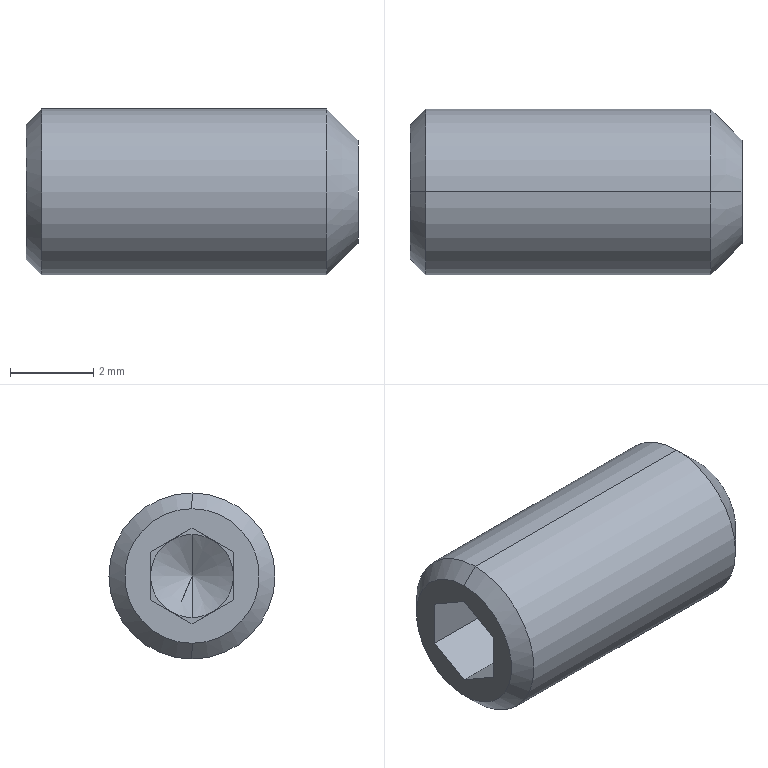Part | SolidWorks | features BaseBody 1 | 1 solid | 22 faces | box 8 x 4 x 4 mm | volume 90.792 mm3 | plane 14 | cone 6 | cylinder 2 | commonest cylinder face diameters 4 x2
STEP:
#1=CARTESIAN_POINT('',(2.077,0.,0.));
#2=VERTEX_POINT('',#1);
#3=CARTESIAN_POINT('',(1.5,0.,1.));
#4=VERTEX_POINT('',#3);
#5=CARTESIAN_POINT('',(2.077,0.,0.));
#6=DIRECTION('',(-0.5,0.,0.866));
#7=VECTOR('',#6,1000.);
#8=LINE('',#5,#7);
#9=EDGE_CURVE('',#2,#4,#8,.T.);
#10=ORIENTED_EDGE('',*,*,#9,.F.);
#11=CARTESIAN_POINT('',(1.5,0.,-1.));
#12=VERTEX_POINT('',#11);
#13=CARTESIAN_POINT('',(2.077,0.,0.));
#14=DIRECTION('',(-0.5,0.,-0.866));
#15=VECTOR('',#14,1000.);
#16=LINE('',#13,#15);
#17=EDGE_CURVE('',#2,#12,#16,.T.);
#18=ORIENTED_EDGE('',*,*,#17,.T.);
#19=CARTESIAN_POINT('',(1.5,-0.5,-0.866));
#20=VERTEX_POINT('',#19);
#21=CARTESIAN_POINT('',(1.5,0.,0.));
#22=DIRECTION('',(-1.,0.,0.));
#23=DIRECTION('',(0.,0.,1.));
#24=AXIS2_PLACEMENT_3D('',#21,#22,#23);
#25=CIRCLE('',#24,1.);
#26=EDGE_CURVE('',#12,#20,#25,.T.);
#27=ORIENTED_EDGE('',*,*,#26,.T.);
#28=CARTESIAN_POINT('',(1.5,-1.,0.));
#29=VERTEX_POINT('',#28);
#30=CARTESIAN_POINT('',(1.5,0.,0.));
#31=DIRECTION('',(-1.,0.,0.));
#32=DIRECTION('',(0.,0.,1.));
#33=AXIS2_PLACEMENT_3D('',#30,#31,#32);
#34=CIRCLE('',#33,1.);
#35=EDGE_CURVE('',#20,#29,#34,.T.);
#36=ORIENTED_EDGE('',*,*,#35,.T.);
#37=CARTESIAN_POINT('',(1.5,-0.5,0.866));
#38=VERTEX_POINT('',#37);
#39=CARTESIAN_POINT('',(1.5,0.,0.));
#40=DIRECTION('',(-1.,0.,0.));
#41=DIRECTION('',(0.,0.,1.));
#42=AXIS2_PLACEMENT_3D('',#39,#40,#41);
#43=CIRCLE('',#42,1.);
#44=EDGE_CURVE('',#29,#38,#43,.T.);
#45=ORIENTED_EDGE('',*,*,#44,.T.);
#46=CARTESIAN_POINT('',(1.5,0.,0.));
#47=DIRECTION('',(-1.,0.,0.));
#48=DIRECTION('',(0.,0.,1.));
#49=AXIS2_PLACEMENT_3D('',#46,#47,#48);
#50=CIRCLE('',#49,1.);
#51=EDGE_CURVE('',#38,#4,#50,.T.);
#52=ORIENTED_EDGE('',*,*,#51,.T.);
#53=EDGE_LOOP('',(#10,#18,#27,#36,#45,#52));
#54=FACE_OUTER_BOUND('',#53,.T.);
#55=CARTESIAN_POINT('',(-997.923,0.,0.));
#56=DIRECTION('',(-1.,0.,0.));
#57=DIRECTION('',(0.,0.,1.));
#58=AXIS2_PLACEMENT_3D('',#55,#56,#57);
#59=CONICAL_SURFACE('',#58,1732.051,1.047);
#60=ADVANCED_FACE('',(#54),#59,.F.);
#61=CARTESIAN_POINT('',(0.,0.,1.621));
#62=VERTEX_POINT('',#61);
#63=CARTESIAN_POINT('',(0.,0.,-1.621));
#64=VERTEX_POINT('',#63);
#65=CARTESIAN_POINT('',(0.,0.,0.));
#66=DIRECTION('',(-1.,0.,0.));
#67=DIRECTION('',(0.,0.,1.));
#68=AXIS2_PLACEMENT_3D('',#65,#66,#67);
#69=CIRCLE('',#68,1.621);
#70=EDGE_CURVE('',#62,#64,#69,.T.);
#71=ORIENTED_EDGE('',*,*,#70,.F.);
#72=CARTESIAN_POINT('',(0.379,0.,2.));
#73=VERTEX_POINT('',#72);
#74=CARTESIAN_POINT('',(0.379,0.,2.));
#75=DIRECTION('',(0.7071,0.,0.7071));
#76=VECTOR('',#75,1000.);
#77=LINE('',#74,#76);
#78=EDGE_CURVE('',#62,#73,#77,.T.);
#79=ORIENTED_EDGE('',*,*,#78,.T.);
#80=CARTESIAN_POINT('',(0.379,0.,-2.));
#81=VERTEX_POINT('',#80);
#82=CARTESIAN_POINT('',(0.379,0.,0.));
#83=DIRECTION('',(-1.,0.,0.));
#84=DIRECTION('',(0.,0.,1.));
#85=AXIS2_PLACEMENT_3D('',#82,#83,#84);
#86=CIRCLE('',#85,2.);
#87=EDGE_CURVE('',#73,#81,#86,.T.);
#88=ORIENTED_EDGE('',*,*,#87,.T.);
#89=CARTESIAN_POINT('',(0.379,0.,-2.));
#90=DIRECTION('',(0.7071,0.,-0.7071));
#91=VECTOR('',#90,1000.);
#92=LINE('',#89,#91);
#93=EDGE_CURVE('',#64,#81,#92,.T.);
#94=ORIENTED_EDGE('',*,*,#93,.F.);
#95=EDGE_LOOP('',(#71,#79,#88,#94));
#96=FACE_OUTER_BOUND('',#95,.T.);
#97=CARTESIAN_POINT('',(0.379,0.,0.));
#98=DIRECTION('',(1.,0.,0.));
#99=DIRECTION('',(0.,0.,-1.));
#100=AXIS2_PLACEMENT_3D('',#97,#98,#99);
#101=CONICAL_SURFACE('',#100,2.,0.7854);
#102=ADVANCED_FACE('',(#96),#101,.T.);
#103=CARTESIAN_POINT('',(7.25,0.,2.));
#104=VERTEX_POINT('',#103);
#105=CARTESIAN_POINT('',(7.25,0.,-2.));
#106=VERTEX_POINT('',#105);
#107=CARTESIAN_POINT('',(7.25,0.,0.));
#108=DIRECTION('',(-1.,0.,0.));
#109=DIRECTION('',(0.,0.,1.));
#110=AXIS2_PLACEMENT_3D('',#107,#108,#109);
#111=CIRCLE('',#110,2.);
#112=EDGE_CURVE('',#104,#106,#111,.T.);
#113=ORIENTED_EDGE('',*,*,#112,.T.);
#114=CARTESIAN_POINT('',(-10.745,0.,-2.));
#115=DIRECTION('',(-1.,0.,0.));
#116=VECTOR('',#115,1000.);
#117=LINE('',#114,#116);
#118=EDGE_CURVE('',#106,#81,#117,.T.);
#119=ORIENTED_EDGE('',*,*,#118,.T.);
#120=ORIENTED_EDGE('',*,*,#87,.F.);
#121=CARTESIAN_POINT('',(-10.745,0.,2.));
#122=DIRECTION('',(-1.,0.,0.));
#123=VECTOR('',#122,1000.);
#124=LINE('',#121,#123);
#125=EDGE_CURVE('',#104,#73,#124,.T.);
#126=ORIENTED_EDGE('',*,*,#125,.F.);
#127=EDGE_LOOP('',(#113,#119,#120,#126));
#128=FACE_OUTER_BOUND('',#127,.T.);
#129=CARTESIAN_POINT('',(-10.745,0.,0.));
#130=DIRECTION('',(-1.,0.,0.));
#131=DIRECTION('',(0.,0.,1.));
#132=AXIS2_PLACEMENT_3D('',#129,#130,#131);
#133=CYLINDRICAL_SURFACE('',#132,2.);
#134=ADVANCED_FACE('',(#128),#133,.T.);
#135=CARTESIAN_POINT('',(8.,0.,1.25));
#136=VERTEX_POINT('',#135);
#137=CARTESIAN_POINT('',(8.,0.,-1.25));
#138=VERTEX_POINT('',#137);
#139=CARTESIAN_POINT('',(8.,0.,0.));
#140=DIRECTION('',(-1.,0.,0.));
#141=DIRECTION('',(0.,0.,1.));
#142=AXIS2_PLACEMENT_3D('',#139,#140,#141);
#143=CIRCLE('',#142,1.25);
#144=EDGE_CURVE('',#136,#138,#143,.T.);
#145=ORIENTED_EDGE('',*,*,#144,.T.);
#146=CARTESIAN_POINT('',(8.,0.,-1.25));
#147=DIRECTION('',(-0.7071,0.,-0.7071));
#148=VECTOR('',#147,1000.);
#149=LINE('',#146,#148);
#150=EDGE_CURVE('',#138,#106,#149,.T.);
#151=ORIENTED_EDGE('',*,*,#150,.T.);
#152=ORIENTED_EDGE('',*,*,#112,.F.);
#153=CARTESIAN_POINT('',(8.,0.,1.25));
#154=DIRECTION('',(-0.7071,0.,0.7071));
#155=VECTOR('',#154,1000.);
#156=LINE('',#153,#155);
#157=EDGE_CURVE('',#136,#104,#156,.T.);
#158=ORIENTED_EDGE('',*,*,#157,.F.);
#159=EDGE_LOOP('',(#145,#151,#152,#158));
#160=FACE_OUTER_BOUND('',#159,.T.);
#161=CARTESIAN_POINT('',(8.,0.,0.));
#162=DIRECTION('',(-1.,0.,0.));
#163=DIRECTION('',(0.,0.,1.));
#164=AXIS2_PLACEMENT_3D('',#161,#162,#163);
#165=CONICAL_SURFACE('',#164,1.25,0.7854);
#166=ADVANCED_FACE('',(#160),#165,.T.);
#167=CARTESIAN_POINT('',(1.5,0.5,0.866));
#168=VERTEX_POINT('',#167);
#169=CARTESIAN_POINT('',(1.5,1.,0.));
#170=VERTEX_POINT('',#169);
#171=CARTESIAN_POINT('',(1.5,0.,0.));
#172=DIRECTION('',(-1.,0.,0.));
#173=DIRECTION('',(0.,0.,1.));
#174=AXIS2_PLACEMENT_3D('',#171,#172,#173);
#175=CIRCLE('',#174,1.);
#176=EDGE_CURVE('',#168,#170,#175,.T.);
#177=ORIENTED_EDGE('',*,*,#176,.F.);
#178=CARTESIAN_POINT('',(1.5,1.,0.5774));
#179=VERTEX_POINT('',#178);
#180=CARTESIAN_POINT('',(1.5,0.,1.155));
#181=DIRECTION('',(0.,0.866,-0.5));
#182=VECTOR('',#181,1000.);
#183=LINE('',#180,#182);
#184=EDGE_CURVE('',#168,#179,#183,.T.);
#185=ORIENTED_EDGE('',*,*,#184,.T.);
#186=CARTESIAN_POINT('',(1.5,1.,0.5774));
#187=DIRECTION('',(0.,0.,-1.));
#188=VECTOR('',#187,1000.);
#189=LINE('',#186,#188);
#190=EDGE_CURVE('',#179,#170,#189,.T.);
#191=ORIENTED_EDGE('',*,*,#190,.T.);
#192=EDGE_LOOP('',(#177,#185,#191));
#193=FACE_OUTER_BOUND('',#192,.T.);
#194=CARTESIAN_POINT('',(1.5,-1.,0.5774));
#195=DIRECTION('',(1.,0.,0.));
#196=DIRECTION('',(0.,1.,0.));
#197=AXIS2_PLACEMENT_3D('',#194,#195,#196);
#198=PLANE('',#197);
#199=ADVANCED_FACE('',(#193),#198,.F.);
#200=CARTESIAN_POINT('',(1.5,0.5,-0.866));
#201=VERTEX_POINT('',#200);
#202=CARTESIAN_POINT('',(1.5,0.,0.));
#203=DIRECTION('',(-1.,0.,0.));
#204=DIRECTION('',(0.,0.,1.));
#205=AXIS2_PLACEMENT_3D('',#202,#203,#204);
#206=CIRCLE('',#205,1.);
#207=EDGE_CURVE('',#170,#201,#206,.T.);
#208=ORIENTED_EDGE('',*,*,#207,.F.);
#209=CARTESIAN_POINT('',(1.5,1.,-0.5774));
#210=VERTEX_POINT('',#209);
#211=CARTESIAN_POINT('',(1.5,1.,0.5774));
#212=DIRECTION('',(0.,0.,-1.));
#213=VECTOR('',#212,1000.);
#214=LINE('',#211,#213);
#215=EDGE_CURVE('',#170,#210,#214,.T.);
#216=ORIENTED_EDGE('',*,*,#215,.T.);
#217=CARTESIAN_POINT('',(1.5,1.,-0.5774));
#218=DIRECTION('',(0.,-0.866,-0.5));
#219=VECTOR('',#218,1000.);
#220=LINE('',#217,#219);
#221=EDGE_CURVE('',#210,#201,#220,.T.);
#222=ORIENTED_EDGE('',*,*,#221,.T.);
#223=EDGE_LOOP('',(#208,#216,#222));
#224=FACE_OUTER_BOUND('',#223,.T.);
#225=CARTESIAN_POINT('',(1.5,-1.,0.5774));
#226=DIRECTION('',(1.,0.,0.));
#227=DIRECTION('',(0.,1.,0.));
#228=AXIS2_PLACEMENT_3D('',#225,#226,#227);
#229=PLANE('',#228);
#230=ADVANCED_FACE('',(#224),#229,.F.);
#231=CARTESIAN_POINT('',(1.5,0.,0.));
#232=DIRECTION('',(-1.,0.,0.));
#233=DIRECTION('',(0.,0.,1.));
#234=AXIS2_PLACEMENT_3D('',#231,#232,#233);
#235=CIRCLE('',#234,1.);
#236=EDGE_CURVE('',#201,#12,#235,.T.);
#237=ORIENTED_EDGE('',*,*,#236,.F.);
#238=CARTESIAN_POINT('',(1.5,0.,-1.155));
#239=VERTEX_POINT('',#238);
#240=CARTESIAN_POINT('',(1.5,1.,-0.5774));
#241=DIRECTION('',(0.,-0.866,-0.5));
#242=VECTOR('',#241,1000.);
#243=LINE('',#240,#242);
#244=EDGE_CURVE('',#201,#239,#243,.T.);
#245=ORIENTED_EDGE('',*,*,#244,.T.);
#246=CARTESIAN_POINT('',(1.5,0.,-1.155));
#247=DIRECTION('',(0.,-0.866,0.5));
#248=VECTOR('',#247,1000.);
#249=LINE('',#246,#248);
#250=EDGE_CURVE('',#239,#20,#249,.T.);
#251=ORIENTED_EDGE('',*,*,#250,.T.);
#252=ORIENTED_EDGE('',*,*,#26,.F.);
#253=EDGE_LOOP('',(#237,#245,#251,#252));
#254=FACE_OUTER_BOUND('',#253,.T.);
#255=CARTESIAN_POINT('',(1.5,-1.,0.5774));
#256=DIRECTION('',(1.,0.,0.));
#257=DIRECTION('',(0.,1.,0.));
#258=AXIS2_PLACEMENT_3D('',#255,#256,#257);
#259=PLANE('',#258);
#260=ADVANCED_FACE('',(#254),#259,.F.);
#261=ORIENTED_EDGE('',*,*,#35,.F.);
#262=CARTESIAN_POINT('',(1.5,-1.,-0.5774));
#263=VERTEX_POINT('',#262);
#264=CARTESIAN_POINT('',(1.5,0.,-1.155));
#265=DIRECTION('',(0.,-0.866,0.5));
#266=VECTOR('',#265,1000.);
#267=LINE('',#264,#266);
#268=EDGE_CURVE('',#20,#263,#267,.T.);
#269=ORIENTED_EDGE('',*,*,#268,.T.);
#270=CARTESIAN_POINT('',(1.5,-1.,-0.5774));
#271=DIRECTION('',(0.,0.,1.));
#272=VECTOR('',#271,1000.);
#273=LINE('',#270,#272);
#274=EDGE_CURVE('',#263,#29,#273,.T.);
#275=ORIENTED_EDGE('',*,*,#274,.T.);
#276=EDGE_LOOP('',(#261,#269,#275));
#277=FACE_OUTER_BOUND('',#276,.T.);
#278=CARTESIAN_POINT('',(1.5,-1.,0.5774));
#279=DIRECTION('',(1.,0.,0.));
#280=DIRECTION('',(0.,1.,0.));
#281=AXIS2_PLACEMENT_3D('',#278,#279,#280);
#282=PLANE('',#281);
#283=ADVANCED_FACE('',(#277),#282,.F.);
#284=ORIENTED_EDGE('',*,*,#44,.F.);
#285=CARTESIAN_POINT('',(1.5,-1.,0.5774));
#286=VERTEX_POINT('',#285);
#287=CARTESIAN_POINT('',(1.5,-1.,-0.5774));
#288=DIRECTION('',(0.,0.,1.));
#289=VECTOR('',#288,1000.);
#290=LINE('',#287,#289);
#291=EDGE_CURVE('',#29,#286,#290,.T.);
#292=ORIENTED_EDGE('',*,*,#291,.T.);
#293=CARTESIAN_POINT('',(1.5,-1.,0.5774));
#294=DIRECTION('',(0.,0.866,0.5));
#295=VECTOR('',#294,1000.);
#296=LINE('',#293,#295);
#297=EDGE_CURVE('',#286,#38,#296,.T.);
#298=ORIENTED_EDGE('',*,*,#297,.T.);
#299=EDGE_LOOP('',(#284,#292,#298));
#300=FACE_OUTER_BOUND('',#299,.T.);
#301=CARTESIAN_POINT('',(1.5,-1.,0.5774));
#302=DIRECTION('',(1.,0.,0.));
#303=DIRECTION('',(0.,1.,0.));
#304=AXIS2_PLACEMENT_3D('',#301,#302,#303);
#305=PLANE('',#304);
#306=ADVANCED_FACE('',(#300),#305,.F.);
#307=ORIENTED_EDGE('',*,*,#51,.F.);
#308=CARTESIAN_POINT('',(1.5,0.,1.155));
#309=VERTEX_POINT('',#308);
#310=CARTESIAN_POINT('',(1.5,-1.,0.5774));
#311=DIRECTION('',(0.,0.866,0.5));
#312=VECTOR('',#311,1000.);
#313=LINE('',#310,#312);
#314=EDGE_CURVE('',#38,#309,#313,.T.);
#315=ORIENTED_EDGE('',*,*,#314,.T.);
#316=CARTESIAN_POINT('',(1.5,0.,1.155));
#317=DIRECTION('',(0.,0.866,-0.5));
#318=VECTOR('',#317,1000.);
#319=LINE('',#316,#318);
#320=EDGE_CURVE('',#309,#168,#319,.T.);
#321=ORIENTED_EDGE('',*,*,#320,.T.);
#322=CARTESIAN_POINT('',(1.5,0.,0.));
#323=DIRECTION('',(-1.,0.,0.));
#324=DIRECTION('',(0.,0.,1.));
#325=AXIS2_PLACEMENT_3D('',#322,#323,#324);
#326=CIRCLE('',#325,1.);
#327=EDGE_CURVE('',#4,#168,#326,.T.);
#328=ORIENTED_EDGE('',*,*,#327,.F.);
#329=EDGE_LOOP('',(#307,#315,#321,#328));
#330=FACE_OUTER_BOUND('',#329,.T.);
#331=CARTESIAN_POINT('',(1.5,-1.,0.5774));
#332=DIRECTION('',(1.,0.,0.));
#333=DIRECTION('',(0.,1.,0.));
#334=AXIS2_PLACEMENT_3D('',#331,#332,#333);
#335=PLANE('',#334);
#336=ADVANCED_FACE('',(#330),#335,.F.);
#337=CARTESIAN_POINT('',(0.,0.,1.155));
#338=VERTEX_POINT('',#337);
#339=CARTESIAN_POINT('',(0.,1.,0.5774));
#340=VERTEX_POINT('',#339);
#341=CARTESIAN_POINT('',(0.,0.,1.155));
#342=DIRECTION('',(0.,0.866,-0.5));
#343=VECTOR('',#342,1000.);
#344=LINE('',#341,#343);
#345=EDGE_CURVE('',#338,#340,#344,.T.);
#346=ORIENTED_EDGE('',*,*,#345,.F.);
#347=CARTESIAN_POINT('',(0.,-1.,0.5774));
#348=VERTEX_POINT('',#347);
#349=CARTESIAN_POINT('',(0.,-1.,0.5774));
#350=DIRECTION('',(0.,0.866,0.5));
#351=VECTOR('',#350,1000.);
#352=LINE('',#349,#351);
#353=EDGE_CURVE('',#348,#338,#352,.T.);
#354=ORIENTED_EDGE('',*,*,#353,.F.);
#355=CARTESIAN_POINT('',(0.,-1.,-0.5774));
#356=VERTEX_POINT('',#355);
#357=CARTESIAN_POINT('',(0.,-1.,-0.5774));
#358=DIRECTION('',(0.,0.,1.));
#359=VECTOR('',#358,1000.);
#360=LINE('',#357,#359);
#361=EDGE_CURVE('',#356,#348,#360,.T.);
#362=ORIENTED_EDGE('',*,*,#361,.F.);
#363=CARTESIAN_POINT('',(0.,0.,-1.155));
#364=VERTEX_POINT('',#363);
#365=CARTESIAN_POINT('',(0.,0.,-1.155));
#366=DIRECTION('',(0.,-0.866,0.5));
#367=VECTOR('',#366,1000.);
#368=LINE('',#365,#367);
#369=EDGE_CURVE('',#364,#356,#368,.T.);
#370=ORIENTED_EDGE('',*,*,#369,.F.);
#371=CARTESIAN_POINT('',(0.,1.,-0.5774));
#372=VERTEX_POINT('',#371);
#373=CARTESIAN_POINT('',(0.,1.,-0.5774));
#374=DIRECTION('',(0.,-0.866,-0.5));
#375=VECTOR('',#374,1000.);
#376=LINE('',#373,#375);
#377=EDGE_CURVE('',#372,#364,#376,.T.);
#378=ORIENTED_EDGE('',*,*,#377,.F.);
#379=CARTESIAN_POINT('',(0.,1.,0.5774));
#380=DIRECTION('',(0.,0.,-1.));
#381=VECTOR('',#380,1000.);
#382=LINE('',#379,#381);
#383=EDGE_CURVE('',#340,#372,#382,.T.);
#384=ORIENTED_EDGE('',*,*,#383,.F.);
#385=EDGE_LOOP('',(#346,#354,#362,#370,#378,#384));
#386=FACE_BOUND('',#385,.T.);
#387=CARTESIAN_POINT('',(0.,0.,0.));
#388=DIRECTION('',(-1.,0.,0.));
#389=DIRECTION('',(0.,0.,1.));
#390=AXIS2_PLACEMENT_3D('',#387,#388,#389);
#391=CIRCLE('',#390,1.621);
#392=EDGE_CURVE('',#64,#62,#391,.T.);
#393=ORIENTED_EDGE('',*,*,#392,.T.);
#394=ORIENTED_EDGE('',*,*,#70,.T.);
#395=EDGE_LOOP('',(#393,#394));
#396=FACE_OUTER_BOUND('',#395,.T.);
#397=CARTESIAN_POINT('',(0.,1.621,0.));
#398=DIRECTION('',(1.,0.,0.));
#399=DIRECTION('',(0.,1.,0.));
#400=AXIS2_PLACEMENT_3D('',#397,#398,#399);
#401=PLANE('',#400);
#402=ADVANCED_FACE('',(#386,#396),#401,.F.);
#403=ORIENTED_EDGE('',*,*,#144,.F.);
#404=CARTESIAN_POINT('',(8.,0.,0.));
#405=DIRECTION('',(-1.,0.,0.));
#406=DIRECTION('',(0.,0.,1.));
#407=AXIS2_PLACEMENT_3D('',#404,#405,#406);
#408=CIRCLE('',#407,1.25);
#409=EDGE_CURVE('',#138,#136,#408,.T.);
#410=ORIENTED_EDGE('',*,*,#409,.F.);
#411=EDGE_LOOP('',(#403,#410));
#412=FACE_OUTER_BOUND('',#411,.T.);
#413=CARTESIAN_POINT('',(8.,0.,0.));
#414=DIRECTION('',(-1.,0.,0.));
#415=DIRECTION('',(0.,0.,1.));
#416=AXIS2_PLACEMENT_3D('',#413,#414,#415);
#417=PLANE('',#416);
#418=ADVANCED_FACE('',(#412),#417,.F.);
#419=ORIENTED_EDGE('',*,*,#150,.F.);
#420=ORIENTED_EDGE('',*,*,#409,.T.);
#421=ORIENTED_EDGE('',*,*,#157,.T.);
#422=CARTESIAN_POINT('',(7.25,0.,0.));
#423=DIRECTION('',(-1.,0.,0.));
#424=DIRECTION('',(0.,0.,1.));
#425=AXIS2_PLACEMENT_3D('',#422,#423,#424);
#426=CIRCLE('',#425,2.);
#427=EDGE_CURVE('',#106,#104,#426,.T.);
#428=ORIENTED_EDGE('',*,*,#427,.F.);
#429=EDGE_LOOP('',(#419,#420,#421,#428));
#430=FACE_OUTER_BOUND('',#429,.T.);
#431=CARTESIAN_POINT('',(8.,0.,0.));
#432=DIRECTION('',(-1.,0.,0.));
#433=DIRECTION('',(0.,0.,1.));
#434=AXIS2_PLACEMENT_3D('',#431,#432,#433);
#435=CONICAL_SURFACE('',#434,1.25,0.7854);
#436=ADVANCED_FACE('',(#430),#435,.T.);
#437=ORIENTED_EDGE('',*,*,#118,.F.);
#438=ORIENTED_EDGE('',*,*,#427,.T.);
#439=ORIENTED_EDGE('',*,*,#125,.T.);
#440=CARTESIAN_POINT('',(0.379,0.,0.));
#441=DIRECTION('',(-1.,0.,0.));
#442=DIRECTION('',(0.,0.,1.));
#443=AXIS2_PLACEMENT_3D('',#440,#441,#442);
#444=CIRCLE('',#443,2.);
#445=EDGE_CURVE('',#81,#73,#444,.T.);
#446=ORIENTED_EDGE('',*,*,#445,.F.);
#447=EDGE_LOOP('',(#437,#438,#439,#446));
#448=FACE_OUTER_BOUND('',#447,.T.);
#449=CARTESIAN_POINT('',(-10.745,0.,0.));
#450=DIRECTION('',(-1.,0.,0.));
#451=DIRECTION('',(0.,0.,1.));
#452=AXIS2_PLACEMENT_3D('',#449,#450,#451);
#453=CYLINDRICAL_SURFACE('',#452,2.);
#454=ADVANCED_FACE('',(#448),#453,.T.);
#455=ORIENTED_EDGE('',*,*,#78,.F.);
#456=ORIENTED_EDGE('',*,*,#392,.F.);
#457=ORIENTED_EDGE('',*,*,#93,.T.);
#458=ORIENTED_EDGE('',*,*,#445,.T.);
#459=EDGE_LOOP('',(#455,#456,#457,#458));
#460=FACE_OUTER_BOUND('',#459,.T.);
#461=CARTESIAN_POINT('',(0.379,0.,0.));
#462=DIRECTION('',(1.,0.,0.));
#463=DIRECTION('',(0.,0.,-1.));
#464=AXIS2_PLACEMENT_3D('',#461,#462,#463);
#465=CONICAL_SURFACE('',#464,2.,0.7854);
#466=ADVANCED_FACE('',(#460),#465,.T.);
#467=ORIENTED_EDGE('',*,*,#353,.T.);
#468=CARTESIAN_POINT('',(1.5,0.,1.155));
#469=DIRECTION('',(-1.,0.,0.));
#470=VECTOR('',#469,1000.);
#471=LINE('',#468,#470);
#472=EDGE_CURVE('',#309,#338,#471,.T.);
#473=ORIENTED_EDGE('',*,*,#472,.F.);
#474=ORIENTED_EDGE('',*,*,#314,.F.);
#475=ORIENTED_EDGE('',*,*,#297,.F.);
#476=CARTESIAN_POINT('',(1.5,-1.,0.5774));
#477=DIRECTION('',(-1.,0.,0.));
#478=VECTOR('',#477,1000.);
#479=LINE('',#476,#478);
#480=EDGE_CURVE('',#286,#348,#479,.T.);
#481=ORIENTED_EDGE('',*,*,#480,.T.);
#482=EDGE_LOOP('',(#467,#473,#474,#475,#481));
#483=FACE_OUTER_BOUND('',#482,.T.);
#484=CARTESIAN_POINT('',(1.5,-1.,0.5774));
#485=DIRECTION('',(0.,-0.5,0.866));
#486=DIRECTION('',(-1.,0.,0.));
#487=AXIS2_PLACEMENT_3D('',#484,#485,#486);
#488=PLANE('',#487);
#489=ADVANCED_FACE('',(#483),#488,.F.);
#490=ORIENTED_EDGE('',*,*,#361,.T.);
#491=ORIENTED_EDGE('',*,*,#480,.F.);
#492=ORIENTED_EDGE('',*,*,#291,.F.);
#493=ORIENTED_EDGE('',*,*,#274,.F.);
#494=CARTESIAN_POINT('',(1.5,-1.,-0.5774));
#495=DIRECTION('',(-1.,0.,0.));
#496=VECTOR('',#495,1000.);
#497=LINE('',#494,#496);
#498=EDGE_CURVE('',#263,#356,#497,.T.);
#499=ORIENTED_EDGE('',*,*,#498,.T.);
#500=EDGE_LOOP('',(#490,#491,#492,#493,#499));
#501=FACE_OUTER_BOUND('',#500,.T.);
#502=CARTESIAN_POINT('',(1.5,-1.,-0.5774));
#503=DIRECTION('',(0.,-1.,0.));
#504=DIRECTION('',(0.,0.,-1.));
#505=AXIS2_PLACEMENT_3D('',#502,#503,#504);
#506=PLANE('',#505);
#507=ADVANCED_FACE('',(#501),#506,.F.);
#508=ORIENTED_EDGE('',*,*,#369,.T.);
#509=ORIENTED_EDGE('',*,*,#498,.F.);
#510=ORIENTED_EDGE('',*,*,#268,.F.);
#511=ORIENTED_EDGE('',*,*,#250,.F.);
#512=CARTESIAN_POINT('',(1.5,0.,-1.155));
#513=DIRECTION('',(-1.,0.,0.));
#514=VECTOR('',#513,1000.);
#515=LINE('',#512,#514);
#516=EDGE_CURVE('',#239,#364,#515,.T.);
#517=ORIENTED_EDGE('',*,*,#516,.T.);
#518=EDGE_LOOP('',(#508,#509,#510,#511,#517));
#519=FACE_OUTER_BOUND('',#518,.T.);
#520=CARTESIAN_POINT('',(1.5,0.,-1.155));
#521=DIRECTION('',(0.,-0.5,-0.866));
#522=DIRECTION('',(0.,-0.866,0.5));
#523=AXIS2_PLACEMENT_3D('',#520,#521,#522);
#524=PLANE('',#523);
#525=ADVANCED_FACE('',(#519),#524,.F.);
#526=ORIENTED_EDGE('',*,*,#377,.T.);
#527=ORIENTED_EDGE('',*,*,#516,.F.);
#528=ORIENTED_EDGE('',*,*,#244,.F.);
#529=ORIENTED_EDGE('',*,*,#221,.F.);
#530=CARTESIAN_POINT('',(1.5,1.,-0.5774));
#531=DIRECTION('',(-1.,0.,0.));
#532=VECTOR('',#531,1000.);
#533=LINE('',#530,#532);
#534=EDGE_CURVE('',#210,#372,#533,.T.);
#535=ORIENTED_EDGE('',*,*,#534,.T.);
#536=EDGE_LOOP('',(#526,#527,#528,#529,#535));
#537=FACE_OUTER_BOUND('',#536,.T.);
#538=CARTESIAN_POINT('',(1.5,1.,-0.5774));
#539=DIRECTION('',(0.,0.5,-0.866));
#540=DIRECTION('',(-1.,0.,0.));
#541=AXIS2_PLACEMENT_3D('',#538,#539,#540);
#542=PLANE('',#541);
#543=ADVANCED_FACE('',(#537),#542,.F.);
#544=ORIENTED_EDGE('',*,*,#383,.T.);
#545=ORIENTED_EDGE('',*,*,#534,.F.);
#546=ORIENTED_EDGE('',*,*,#215,.F.);
#547=ORIENTED_EDGE('',*,*,#190,.F.);
#548=CARTESIAN_POINT('',(1.5,1.,0.5774));
#549=DIRECTION('',(-1.,0.,0.));
#550=VECTOR('',#549,1000.);
#551=LINE('',#548,#550);
#552=EDGE_CURVE('',#179,#340,#551,.T.);
#553=ORIENTED_EDGE('',*,*,#552,.T.);
#554=EDGE_LOOP('',(#544,#545,#546,#547,#553));
#555=FACE_OUTER_BOUND('',#554,.T.);
#556=CARTESIAN_POINT('',(1.5,1.,0.5774));
#557=DIRECTION('',(0.,1.,0.));
#558=DIRECTION('',(1.,0.,0.));
#559=AXIS2_PLACEMENT_3D('',#556,#557,#558);
#560=PLANE('',#559);
#561=ADVANCED_FACE('',(#555),#560,.F.);
#562=ORIENTED_EDGE('',*,*,#345,.T.);
#563=ORIENTED_EDGE('',*,*,#552,.F.);
#564=ORIENTED_EDGE('',*,*,#184,.F.);
#565=ORIENTED_EDGE('',*,*,#320,.F.);
#566=ORIENTED_EDGE('',*,*,#472,.T.);
#567=EDGE_LOOP('',(#562,#563,#564,#565,#566));
#568=FACE_OUTER_BOUND('',#567,.T.);
#569=CARTESIAN_POINT('',(1.5,0.,1.155));
#570=DIRECTION('',(0.,0.5,0.866));
#571=DIRECTION('',(1.,0.,0.));
#572=AXIS2_PLACEMENT_3D('',#569,#570,#571);
#573=PLANE('',#572);
#574=ADVANCED_FACE('',(#568),#573,.F.);
#575=ORIENTED_EDGE('',*,*,#17,.F.);
#576=ORIENTED_EDGE('',*,*,#9,.T.);
#577=ORIENTED_EDGE('',*,*,#327,.T.);
#578=ORIENTED_EDGE('',*,*,#176,.T.);
#579=ORIENTED_EDGE('',*,*,#207,.T.);
#580=ORIENTED_EDGE('',*,*,#236,.T.);
#581=EDGE_LOOP('',(#575,#576,#577,#578,#579,#580));
#582=FACE_OUTER_BOUND('',#581,.T.);
#583=CARTESIAN_POINT('',(-997.923,0.,0.));
#584=DIRECTION('',(-1.,0.,0.));
#585=DIRECTION('',(0.,0.,1.));
#586=AXIS2_PLACEMENT_3D('',#583,#584,#585);
#587=CONICAL_SURFACE('',#586,1732.051,1.047);
#588=ADVANCED_FACE('',(#582),#587,.F.);
#589=CLOSED_SHELL('',(#60,#102,#134,#166,#199,#230,#260,#283,#306,#336,#402,#418,#436,#454,#466,#489,#507,#525,#543,#561,#574,#588));
#590=MANIFOLD_SOLID_BREP('',#589);
#591=CARTESIAN_POINT('',(0.,0.,0.));
#592=DIRECTION('',(0.,0.,1.));
#593=DIRECTION('',(1.,0.,0.));
#594=AXIS2_PLACEMENT_3D('',#591,#592,#593);
#595=(LENGTH_UNIT()NAMED_UNIT(*)SI_UNIT(.MILLI.,.METRE.));
#596=UNCERTAINTY_MEASURE_WITH_UNIT(LENGTH_MEASURE(0.00001),#595,'','');
#597=(NAMED_UNIT(*)PLANE_ANGLE_UNIT()SI_UNIT($,.RADIAN.));
#598=(NAMED_UNIT(*)SI_UNIT($,.STERADIAN.)SOLID_ANGLE_UNIT());
#599=(GEOMETRIC_REPRESENTATION_CONTEXT(3)GLOBAL_UNCERTAINTY_ASSIGNED_CONTEXT((#596))GLOBAL_UNIT_ASSIGNED_CONTEXT((#595,#597,#598))REPRESENTATION_CONTEXT('',''));
#600=ADVANCED_BREP_SHAPE_REPRESENTATION('',(#590,#594),#599);